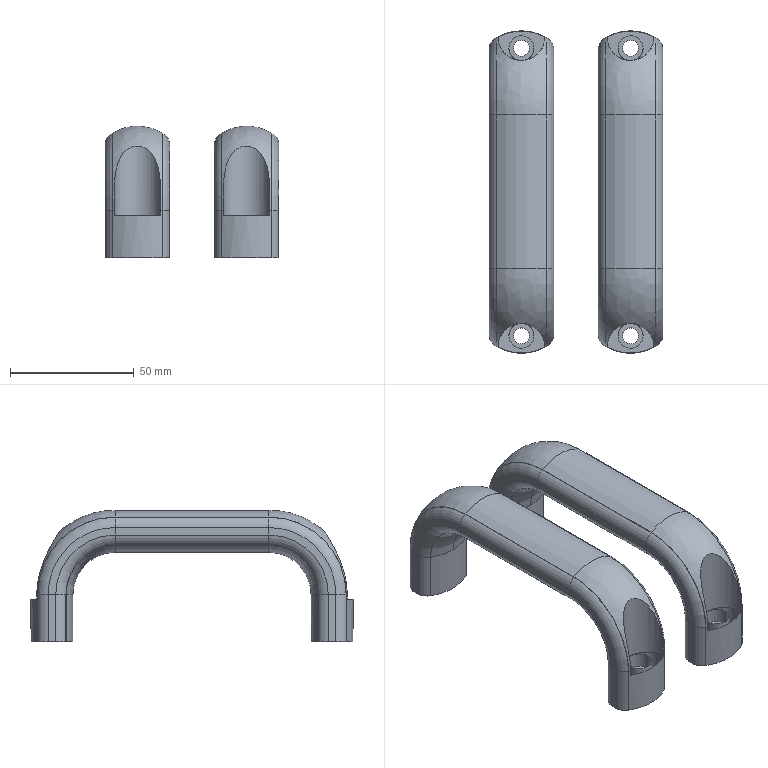Part | SolidWorks | 2 solids | 156 faces | box 70 x 130 x 53 mm | volume 112751 mm3 | cylinder 80 | torus 40 | plane 32 | spline 4 | commonest cylinder face diameters 11.333 x24 20 x24 39.767 x12 6.4 x8 10.1 x8 18.898 x4